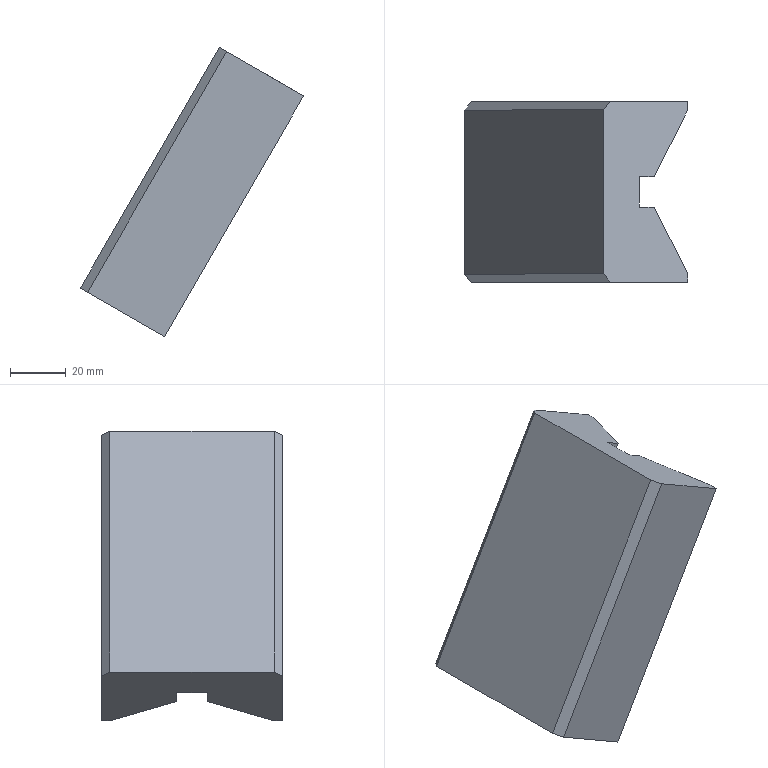Part | NX | features solid 2 | 1 solid | 14 faces | box 80.311 x 65 x 104.103 mm | volume 171497 mm3 | plane 14
STEP:
#1=CARTESIAN_POINT('',(294.401,-157.5,17.982));
#2=VERTEX_POINT('',#1);
#3=CARTESIAN_POINT('',(266.688,-157.5,33.982));
#4=VERTEX_POINT('',#3);
#5=CARTESIAN_POINT('',(294.401,-157.5,17.982));
#6=DIRECTION('',(-0.866,0.,0.5));
#7=VECTOR('',#6,1000.);
#8=LINE('',#5,#7);
#9=EDGE_CURVE('',#2,#4,#8,.T.);
#10=ORIENTED_EDGE('',*,*,#9,.T.);
#11=CARTESIAN_POINT('',(264.09,-160.5,35.482));
#12=VERTEX_POINT('',#11);
#13=CARTESIAN_POINT('',(266.472,-157.75,34.107));
#14=DIRECTION('',(0.6124,0.7071,-0.3536));
#15=VECTOR('',#14,1000.);
#16=LINE('',#13,#15);
#17=EDGE_CURVE('',#4,#12,#16,.F.);
#18=ORIENTED_EDGE('',*,*,#17,.T.);
#19=CARTESIAN_POINT('',(264.09,-219.5,35.482));
#20=VERTEX_POINT('',#19);
#21=CARTESIAN_POINT('',(264.09,-190.,35.482));
#22=DIRECTION('',(0.,-1.,0.));
#23=VECTOR('',#22,1000.);
#24=LINE('',#21,#23);
#25=EDGE_CURVE('',#12,#20,#24,.T.);
#26=ORIENTED_EDGE('',*,*,#25,.T.);
#27=CARTESIAN_POINT('',(266.688,-222.5,33.982));
#28=VERTEX_POINT('',#27);
#29=CARTESIAN_POINT('',(266.472,-222.25,34.107));
#30=DIRECTION('',(-0.6124,0.7071,0.3536));
#31=VECTOR('',#30,1000.);
#32=LINE('',#29,#31);
#33=EDGE_CURVE('',#20,#28,#32,.F.);
#34=ORIENTED_EDGE('',*,*,#33,.T.);
#35=CARTESIAN_POINT('',(294.401,-222.5,17.982));
#36=VERTEX_POINT('',#35);
#37=CARTESIAN_POINT('',(294.401,-222.5,17.982));
#38=DIRECTION('',(-0.866,0.,0.5));
#39=VECTOR('',#38,1000.);
#40=LINE('',#37,#39);
#41=EDGE_CURVE('',#36,#28,#40,.T.);
#42=ORIENTED_EDGE('',*,*,#41,.F.);
#43=CARTESIAN_POINT('',(294.401,-219.445,17.982));
#44=VERTEX_POINT('',#43);
#45=CARTESIAN_POINT('',(294.401,-190.,17.982));
#46=DIRECTION('',(0.,1.,0.));
#47=VECTOR('',#46,1000.);
#48=LINE('',#45,#47);
#49=EDGE_CURVE('',#36,#44,#48,.T.);
#50=ORIENTED_EDGE('',*,*,#49,.T.);
#51=CARTESIAN_POINT('',(282.429,-195.5,24.894));
#52=VERTEX_POINT('',#51);
#53=CARTESIAN_POINT('',(283.359,-197.361,24.357));
#54=DIRECTION('',(-0.433,0.866,0.25));
#55=VECTOR('',#54,1000.);
#56=LINE('',#53,#55);
#57=EDGE_CURVE('',#44,#52,#56,.T.);
#58=ORIENTED_EDGE('',*,*,#57,.T.);
#59=CARTESIAN_POINT('',(277.081,-195.5,27.982));
#60=VERTEX_POINT('',#59);
#61=CARTESIAN_POINT('',(294.401,-195.5,17.982));
#62=DIRECTION('',(0.866,0.,-0.5));
#63=VECTOR('',#62,1000.);
#64=LINE('',#61,#63);
#65=EDGE_CURVE('',#52,#60,#64,.F.);
#66=ORIENTED_EDGE('',*,*,#65,.T.);
#67=CARTESIAN_POINT('',(277.081,-184.5,27.982));
#68=VERTEX_POINT('',#67);
#69=CARTESIAN_POINT('',(277.081,-190.,27.982));
#70=DIRECTION('',(0.,-1.,0.));
#71=VECTOR('',#70,1000.);
#72=LINE('',#69,#71);
#73=EDGE_CURVE('',#68,#60,#72,.T.);
#74=ORIENTED_EDGE('',*,*,#73,.F.);
#75=CARTESIAN_POINT('',(282.429,-184.5,24.894));
#76=VERTEX_POINT('',#75);
#77=CARTESIAN_POINT('',(294.401,-184.5,17.982));
#78=DIRECTION('',(0.866,0.,-0.5));
#79=VECTOR('',#78,1000.);
#80=LINE('',#77,#79);
#81=EDGE_CURVE('',#68,#76,#80,.T.);
#82=ORIENTED_EDGE('',*,*,#81,.T.);
#83=CARTESIAN_POINT('',(294.401,-160.555,17.982));
#84=VERTEX_POINT('',#83);
#85=CARTESIAN_POINT('',(283.359,-182.639,24.357));
#86=DIRECTION('',(-0.433,-0.866,0.25));
#87=VECTOR('',#86,1000.);
#88=LINE('',#85,#87);
#89=EDGE_CURVE('',#84,#76,#88,.T.);
#90=ORIENTED_EDGE('',*,*,#89,.F.);
#91=CARTESIAN_POINT('',(294.401,-190.,17.982));
#92=DIRECTION('',(0.,1.,0.));
#93=VECTOR('',#92,1000.);
#94=LINE('',#91,#93);
#95=EDGE_CURVE('',#84,#2,#94,.T.);
#96=ORIENTED_EDGE('',*,*,#95,.T.);
#97=EDGE_LOOP('',(#10,#18,#26,#34,#42,#50,#58,#66,#74,#82,#90,#96));
#98=FACE_BOUND('',#97,.T.);
#99=CARTESIAN_POINT('',(294.401,-190.,17.982));
#100=DIRECTION('',(0.5,0.,0.866));
#101=DIRECTION('',(-0.866,0.,0.5));
#102=AXIS2_PLACEMENT_3D('',#99,#100,#101);
#103=PLANE('',#102);
#104=ADVANCED_FACE('',(#98),#103,.T.);
#105=CARTESIAN_POINT('',(214.09,-219.5,-51.12));
#106=VERTEX_POINT('',#105);
#107=CARTESIAN_POINT('',(214.09,-160.5,-51.12));
#108=VERTEX_POINT('',#107);
#109=CARTESIAN_POINT('',(214.09,-190.,-51.12));
#110=DIRECTION('',(0.,1.,0.));
#111=VECTOR('',#110,1000.);
#112=LINE('',#109,#111);
#113=EDGE_CURVE('',#106,#108,#112,.T.);
#114=ORIENTED_EDGE('',*,*,#113,.T.);
#115=CARTESIAN_POINT('',(216.688,-157.5,-52.62));
#116=VERTEX_POINT('',#115);
#117=CARTESIAN_POINT('',(216.472,-157.75,-52.495));
#118=DIRECTION('',(-0.6124,-0.7071,0.3536));
#119=VECTOR('',#118,1000.);
#120=LINE('',#117,#119);
#121=EDGE_CURVE('',#108,#116,#120,.F.);
#122=ORIENTED_EDGE('',*,*,#121,.T.);
#123=CARTESIAN_POINT('',(244.401,-157.5,-68.62));
#124=VERTEX_POINT('',#123);
#125=CARTESIAN_POINT('',(244.401,-157.5,-68.62));
#126=DIRECTION('',(-0.866,0.,0.5));
#127=VECTOR('',#126,1000.);
#128=LINE('',#125,#127);
#129=EDGE_CURVE('',#124,#116,#128,.T.);
#130=ORIENTED_EDGE('',*,*,#129,.F.);
#131=CARTESIAN_POINT('',(244.401,-160.555,-68.62));
#132=VERTEX_POINT('',#131);
#133=CARTESIAN_POINT('',(244.401,-190.,-68.62));
#134=DIRECTION('',(0.,-1.,0.));
#135=VECTOR('',#134,1000.);
#136=LINE('',#133,#135);
#137=EDGE_CURVE('',#124,#132,#136,.T.);
#138=ORIENTED_EDGE('',*,*,#137,.T.);
#139=CARTESIAN_POINT('',(232.429,-184.5,-61.708));
#140=VERTEX_POINT('',#139);
#141=CARTESIAN_POINT('',(233.359,-182.639,-62.245));
#142=DIRECTION('',(0.433,0.866,-0.25));
#143=VECTOR('',#142,1000.);
#144=LINE('',#141,#143);
#145=EDGE_CURVE('',#140,#132,#144,.T.);
#146=ORIENTED_EDGE('',*,*,#145,.F.);
#147=CARTESIAN_POINT('',(227.081,-184.5,-58.62));
#148=VERTEX_POINT('',#147);
#149=CARTESIAN_POINT('',(244.401,-184.5,-68.62));
#150=DIRECTION('',(-0.866,0.,0.5));
#151=VECTOR('',#150,1000.);
#152=LINE('',#149,#151);
#153=EDGE_CURVE('',#140,#148,#152,.T.);
#154=ORIENTED_EDGE('',*,*,#153,.T.);
#155=CARTESIAN_POINT('',(227.081,-195.5,-58.62));
#156=VERTEX_POINT('',#155);
#157=CARTESIAN_POINT('',(227.081,-190.,-58.62));
#158=DIRECTION('',(0.,1.,0.));
#159=VECTOR('',#158,1000.);
#160=LINE('',#157,#159);
#161=EDGE_CURVE('',#156,#148,#160,.T.);
#162=ORIENTED_EDGE('',*,*,#161,.F.);
#163=CARTESIAN_POINT('',(232.429,-195.5,-61.708));
#164=VERTEX_POINT('',#163);
#165=CARTESIAN_POINT('',(244.401,-195.5,-68.62));
#166=DIRECTION('',(-0.866,0.,0.5));
#167=VECTOR('',#166,1000.);
#168=LINE('',#165,#167);
#169=EDGE_CURVE('',#156,#164,#168,.F.);
#170=ORIENTED_EDGE('',*,*,#169,.T.);
#171=CARTESIAN_POINT('',(244.401,-219.445,-68.62));
#172=VERTEX_POINT('',#171);
#173=CARTESIAN_POINT('',(233.359,-197.361,-62.245));
#174=DIRECTION('',(0.433,-0.866,-0.25));
#175=VECTOR('',#174,1000.);
#176=LINE('',#173,#175);
#177=EDGE_CURVE('',#164,#172,#176,.T.);
#178=ORIENTED_EDGE('',*,*,#177,.T.);
#179=CARTESIAN_POINT('',(244.401,-222.5,-68.62));
#180=VERTEX_POINT('',#179);
#181=CARTESIAN_POINT('',(244.401,-190.,-68.62));
#182=DIRECTION('',(0.,-1.,0.));
#183=VECTOR('',#182,1000.);
#184=LINE('',#181,#183);
#185=EDGE_CURVE('',#172,#180,#184,.T.);
#186=ORIENTED_EDGE('',*,*,#185,.T.);
#187=CARTESIAN_POINT('',(216.688,-222.5,-52.62));
#188=VERTEX_POINT('',#187);
#189=CARTESIAN_POINT('',(244.401,-222.5,-68.62));
#190=DIRECTION('',(-0.866,0.,0.5));
#191=VECTOR('',#190,1000.);
#192=LINE('',#189,#191);
#193=EDGE_CURVE('',#180,#188,#192,.T.);
#194=ORIENTED_EDGE('',*,*,#193,.T.);
#195=CARTESIAN_POINT('',(216.472,-222.25,-52.495));
#196=DIRECTION('',(0.6124,-0.7071,-0.3536));
#197=VECTOR('',#196,1000.);
#198=LINE('',#195,#197);
#199=EDGE_CURVE('',#188,#106,#198,.F.);
#200=ORIENTED_EDGE('',*,*,#199,.T.);
#201=EDGE_LOOP('',(#114,#122,#130,#138,#146,#154,#162,#170,#178,#186,#194,#200));
#202=FACE_BOUND('',#201,.T.);
#203=CARTESIAN_POINT('',(244.401,-190.,-68.62));
#204=DIRECTION('',(-0.5,0.,-0.866));
#205=DIRECTION('',(0.866,0.,-0.5));
#206=AXIS2_PLACEMENT_3D('',#203,#204,#205);
#207=PLANE('',#206);
#208=ADVANCED_FACE('',(#202),#207,.T.);
#209=ORIENTED_EDGE('',*,*,#177,.F.);
#210=CARTESIAN_POINT('',(294.929,-195.5,46.545));
#211=DIRECTION('',(-0.5,0.,-0.866));
#212=VECTOR('',#211,1000.);
#213=LINE('',#210,#212);
#214=EDGE_CURVE('',#164,#52,#213,.F.);
#215=ORIENTED_EDGE('',*,*,#214,.T.);
#216=ORIENTED_EDGE('',*,*,#57,.F.);
#217=CARTESIAN_POINT('',(269.401,-219.445,-25.319));
#218=DIRECTION('',(0.5,0.,0.866));
#219=VECTOR('',#218,1000.);
#220=LINE('',#217,#219);
#221=EDGE_CURVE('',#172,#44,#220,.T.);
#222=ORIENTED_EDGE('',*,*,#221,.F.);
#223=EDGE_LOOP('',(#209,#215,#216,#222));
#224=FACE_BOUND('',#223,.T.);
#225=CARTESIAN_POINT('',(292.179,-190.,48.133));
#226=DIRECTION('',(0.75,0.5,-0.433));
#227=DIRECTION('',(0.433,-0.866,-0.25));
#228=AXIS2_PLACEMENT_3D('',#225,#226,#227);
#229=PLANE('',#228);
#230=ADVANCED_FACE('',(#224),#229,.T.);
#231=CARTESIAN_POINT('',(294.929,-184.5,46.545));
#232=DIRECTION('',(0.5,0.,0.866));
#233=VECTOR('',#232,1000.);
#234=LINE('',#231,#233);
#235=EDGE_CURVE('',#140,#76,#234,.T.);
#236=ORIENTED_EDGE('',*,*,#235,.F.);
#237=ORIENTED_EDGE('',*,*,#145,.T.);
#238=CARTESIAN_POINT('',(269.401,-160.555,-25.319));
#239=DIRECTION('',(0.5,0.,0.866));
#240=VECTOR('',#239,1000.);
#241=LINE('',#238,#240);
#242=EDGE_CURVE('',#132,#84,#241,.T.);
#243=ORIENTED_EDGE('',*,*,#242,.T.);
#244=ORIENTED_EDGE('',*,*,#89,.T.);
#245=EDGE_LOOP('',(#236,#237,#243,#244));
#246=FACE_BOUND('',#245,.T.);
#247=CARTESIAN_POINT('',(292.179,-190.,48.133));
#248=DIRECTION('',(-0.75,0.5,0.433));
#249=DIRECTION('',(0.433,0.866,-0.25));
#250=AXIS2_PLACEMENT_3D('',#247,#248,#249);
#251=PLANE('',#250);
#252=ADVANCED_FACE('',(#246),#251,.F.);
#253=ORIENTED_EDGE('',*,*,#185,.F.);
#254=ORIENTED_EDGE('',*,*,#221,.T.);
#255=ORIENTED_EDGE('',*,*,#49,.F.);
#256=CARTESIAN_POINT('',(269.401,-222.5,-25.319));
#257=DIRECTION('',(0.5,0.,0.866));
#258=VECTOR('',#257,1000.);
#259=LINE('',#256,#258);
#260=EDGE_CURVE('',#180,#36,#259,.T.);
#261=ORIENTED_EDGE('',*,*,#260,.F.);
#262=EDGE_LOOP('',(#253,#254,#255,#261));
#263=FACE_BOUND('',#262,.T.);
#264=CARTESIAN_POINT('',(269.401,-190.,-25.319));
#265=DIRECTION('',(0.866,0.,-0.5));
#266=DIRECTION('',(0.5,0.,0.866));
#267=AXIS2_PLACEMENT_3D('',#264,#265,#266);
#268=PLANE('',#267);
#269=ADVANCED_FACE('',(#263),#268,.T.);
#270=ORIENTED_EDGE('',*,*,#25,.F.);
#271=CARTESIAN_POINT('',(239.09,-160.5,-7.819));
#272=DIRECTION('',(-0.5,0.,-0.866));
#273=VECTOR('',#272,1000.);
#274=LINE('',#271,#273);
#275=EDGE_CURVE('',#12,#108,#274,.T.);
#276=ORIENTED_EDGE('',*,*,#275,.T.);
#277=ORIENTED_EDGE('',*,*,#113,.F.);
#278=CARTESIAN_POINT('',(239.09,-219.5,-7.819));
#279=DIRECTION('',(0.5,0.,0.866));
#280=VECTOR('',#279,1000.);
#281=LINE('',#278,#280);
#282=EDGE_CURVE('',#106,#20,#281,.T.);
#283=ORIENTED_EDGE('',*,*,#282,.T.);
#284=EDGE_LOOP('',(#270,#276,#277,#283));
#285=FACE_BOUND('',#284,.T.);
#286=CARTESIAN_POINT('',(239.09,-190.,-7.819));
#287=DIRECTION('',(-0.866,0.,0.5));
#288=DIRECTION('',(-0.5,0.,-0.866));
#289=AXIS2_PLACEMENT_3D('',#286,#287,#288);
#290=PLANE('',#289);
#291=ADVANCED_FACE('',(#285),#290,.T.);
#292=ORIENTED_EDGE('',*,*,#129,.T.);
#293=CARTESIAN_POINT('',(241.688,-157.5,-9.319));
#294=DIRECTION('',(0.5,0.,0.866));
#295=VECTOR('',#294,1000.);
#296=LINE('',#293,#295);
#297=EDGE_CURVE('',#116,#4,#296,.T.);
#298=ORIENTED_EDGE('',*,*,#297,.T.);
#299=ORIENTED_EDGE('',*,*,#9,.F.);
#300=CARTESIAN_POINT('',(269.401,-157.5,-25.319));
#301=DIRECTION('',(-0.5,0.,-0.866));
#302=VECTOR('',#301,1000.);
#303=LINE('',#300,#302);
#304=EDGE_CURVE('',#2,#124,#303,.T.);
#305=ORIENTED_EDGE('',*,*,#304,.T.);
#306=EDGE_LOOP('',(#292,#298,#299,#305));
#307=FACE_BOUND('',#306,.T.);
#308=CARTESIAN_POINT('',(269.401,-157.5,-25.319));
#309=DIRECTION('',(0.,1.,0.));
#310=DIRECTION('',(0.866,0.,-0.5));
#311=AXIS2_PLACEMENT_3D('',#308,#309,#310);
#312=PLANE('',#311);
#313=ADVANCED_FACE('',(#307),#312,.T.);
#314=ORIENTED_EDGE('',*,*,#41,.T.);
#315=CARTESIAN_POINT('',(241.688,-222.5,-9.319));
#316=DIRECTION('',(-0.5,0.,-0.866));
#317=VECTOR('',#316,1000.);
#318=LINE('',#315,#317);
#319=EDGE_CURVE('',#28,#188,#318,.T.);
#320=ORIENTED_EDGE('',*,*,#319,.T.);
#321=ORIENTED_EDGE('',*,*,#193,.F.);
#322=ORIENTED_EDGE('',*,*,#260,.T.);
#323=EDGE_LOOP('',(#314,#320,#321,#322));
#324=FACE_BOUND('',#323,.T.);
#325=CARTESIAN_POINT('',(269.401,-222.5,-25.319));
#326=DIRECTION('',(0.,-1.,0.));
#327=DIRECTION('',(-0.866,0.,0.5));
#328=AXIS2_PLACEMENT_3D('',#325,#326,#327);
#329=PLANE('',#328);
#330=ADVANCED_FACE('',(#324),#329,.T.);
#331=ORIENTED_EDGE('',*,*,#242,.F.);
#332=ORIENTED_EDGE('',*,*,#137,.F.);
#333=ORIENTED_EDGE('',*,*,#304,.F.);
#334=ORIENTED_EDGE('',*,*,#95,.F.);
#335=EDGE_LOOP('',(#331,#332,#333,#334));
#336=FACE_BOUND('',#335,.T.);
#337=CARTESIAN_POINT('',(269.401,-190.,-25.319));
#338=DIRECTION('',(0.866,0.,-0.5));
#339=DIRECTION('',(0.5,0.,0.866));
#340=AXIS2_PLACEMENT_3D('',#337,#338,#339);
#341=PLANE('',#340);
#342=ADVANCED_FACE('',(#336),#341,.T.);
#343=ORIENTED_EDGE('',*,*,#214,.F.);
#344=ORIENTED_EDGE('',*,*,#169,.F.);
#345=CARTESIAN_POINT('',(39.581,-195.5,-383.38));
#346=DIRECTION('',(0.5,0.,0.866));
#347=VECTOR('',#346,1000.);
#348=LINE('',#345,#347);
#349=EDGE_CURVE('',#156,#60,#348,.T.);
#350=ORIENTED_EDGE('',*,*,#349,.T.);
#351=ORIENTED_EDGE('',*,*,#65,.F.);
#352=EDGE_LOOP('',(#343,#344,#350,#351));
#353=FACE_BOUND('',#352,.T.);
#354=CARTESIAN_POINT('',(39.581,-195.5,-383.38));
#355=DIRECTION('',(0.,-1.,0.));
#356=DIRECTION('',(0.5,0.,0.866));
#357=AXIS2_PLACEMENT_3D('',#354,#355,#356);
#358=PLANE('',#357);
#359=ADVANCED_FACE('',(#353),#358,.F.);
#360=CARTESIAN_POINT('',(39.581,-184.5,-383.38));
#361=DIRECTION('',(0.5,0.,0.866));
#362=VECTOR('',#361,1000.);
#363=LINE('',#360,#362);
#364=EDGE_CURVE('',#148,#68,#363,.T.);
#365=ORIENTED_EDGE('',*,*,#364,.F.);
#366=ORIENTED_EDGE('',*,*,#153,.F.);
#367=ORIENTED_EDGE('',*,*,#235,.T.);
#368=ORIENTED_EDGE('',*,*,#81,.F.);
#369=EDGE_LOOP('',(#365,#366,#367,#368));
#370=FACE_BOUND('',#369,.T.);
#371=CARTESIAN_POINT('',(39.581,-184.5,-383.38));
#372=DIRECTION('',(0.,-1.,0.));
#373=DIRECTION('',(0.5,0.,0.866));
#374=AXIS2_PLACEMENT_3D('',#371,#372,#373);
#375=PLANE('',#374);
#376=ADVANCED_FACE('',(#370),#375,.T.);
#377=ORIENTED_EDGE('',*,*,#73,.T.);
#378=ORIENTED_EDGE('',*,*,#349,.F.);
#379=ORIENTED_EDGE('',*,*,#161,.T.);
#380=ORIENTED_EDGE('',*,*,#364,.T.);
#381=EDGE_LOOP('',(#377,#378,#379,#380));
#382=FACE_BOUND('',#381,.T.);
#383=CARTESIAN_POINT('',(39.581,-184.5,-383.38));
#384=DIRECTION('',(-0.866,0.,0.5));
#385=DIRECTION('',(-0.5,0.,-0.866));
#386=AXIS2_PLACEMENT_3D('',#383,#384,#385);
#387=PLANE('',#386);
#388=ADVANCED_FACE('',(#382),#387,.F.);
#389=ORIENTED_EDGE('',*,*,#121,.F.);
#390=ORIENTED_EDGE('',*,*,#275,.F.);
#391=ORIENTED_EDGE('',*,*,#17,.F.);
#392=ORIENTED_EDGE('',*,*,#297,.F.);
#393=EDGE_LOOP('',(#389,#390,#391,#392));
#394=FACE_BOUND('',#393,.T.);
#395=CARTESIAN_POINT('',(241.688,-157.5,-9.319));
#396=DIRECTION('',(0.6124,-0.7071,-0.3536));
#397=DIRECTION('',(-0.6124,-0.7071,0.3536));
#398=AXIS2_PLACEMENT_3D('',#395,#396,#397);
#399=PLANE('',#398);
#400=ADVANCED_FACE('',(#394),#399,.F.);
#401=ORIENTED_EDGE('',*,*,#33,.F.);
#402=ORIENTED_EDGE('',*,*,#282,.F.);
#403=ORIENTED_EDGE('',*,*,#199,.F.);
#404=ORIENTED_EDGE('',*,*,#319,.F.);
#405=EDGE_LOOP('',(#401,#402,#403,#404));
#406=FACE_BOUND('',#405,.T.);
#407=CARTESIAN_POINT('',(241.688,-222.5,-9.319));
#408=DIRECTION('',(0.6124,0.7071,-0.3536));
#409=DIRECTION('',(0.6124,-0.7071,-0.3536));
#410=AXIS2_PLACEMENT_3D('',#407,#408,#409);
#411=PLANE('',#410);
#412=ADVANCED_FACE('',(#406),#411,.F.);
#413=CLOSED_SHELL('',(#104,#208,#230,#252,#269,#291,#313,#330,#342,#359,#376,#388,#400,#412));
#414=MANIFOLD_SOLID_BREP('',#413);
#415=(LENGTH_UNIT()NAMED_UNIT(*)SI_UNIT(.MILLI.,.METRE.));
#416=UNCERTAINTY_MEASURE_WITH_UNIT(LENGTH_MEASURE(0.00001),#415,'','');
#417=(NAMED_UNIT(*)PLANE_ANGLE_UNIT()SI_UNIT($,.RADIAN.));
#418=(NAMED_UNIT(*)SI_UNIT($,.STERADIAN.)SOLID_ANGLE_UNIT());
#419=(GEOMETRIC_REPRESENTATION_CONTEXT(3)GLOBAL_UNCERTAINTY_ASSIGNED_CONTEXT((#416))GLOBAL_UNIT_ASSIGNED_CONTEXT((#415,#417,#418))REPRESENTATION_CONTEXT('',''));
#420=ADVANCED_BREP_SHAPE_REPRESENTATION('',(#414),#419);